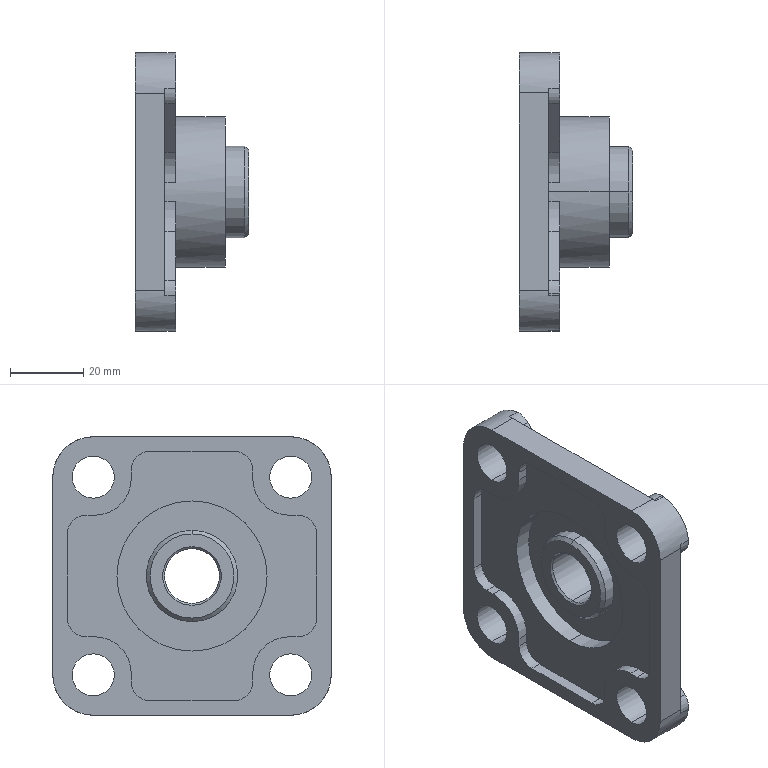Part | SolidWorks | features BaseBody 1 | 1 solid | 117 faces | box 30.9 x 76 x 76 mm | volume 51262 mm3 | cylinder 60 | plane 41 | cone 16 | commonest cylinder face diameters 10 x18 20 x14 11.5 x8 22 x4 25 x4 41 x4